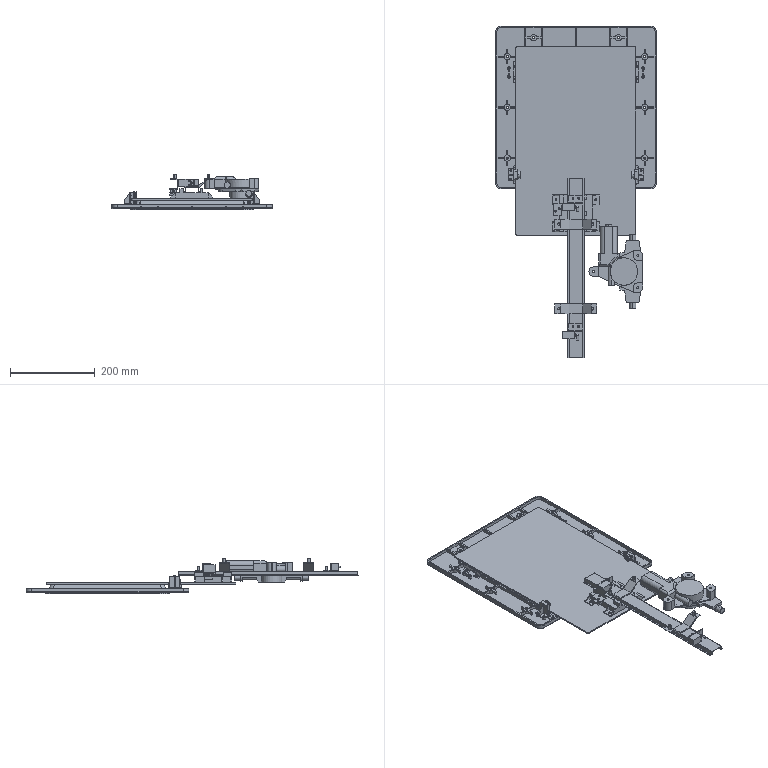Part | SolidWorks | features BaseBody 24, RefSurface 1 | 21 solids | 1211 faces | box 380 x 785.607 x 83.5 mm | volume 1277460 mm3 | plane 681 | cylinder 408 | torus 70 | cone 28 | spline 24 | commonest cylinder face diameters 5 x50 7 x40 15 x34 4 x28 2 x26 3 x24